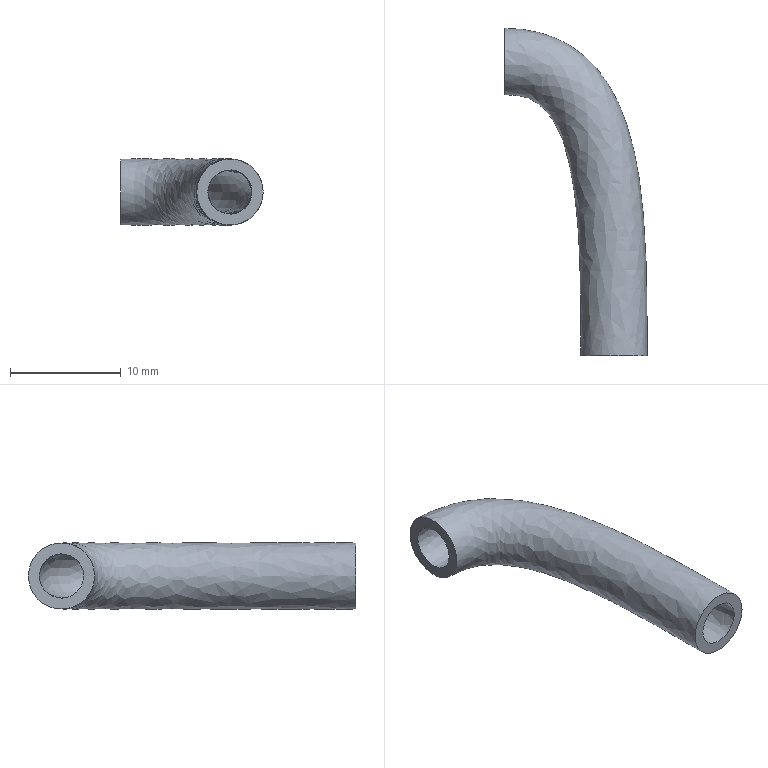Part | NX | features solid 2 | 1 solid | 4 faces | box 12.875 x 29.614 x 6 mm | volume 495.282 mm3 | plane 2 | spline 2